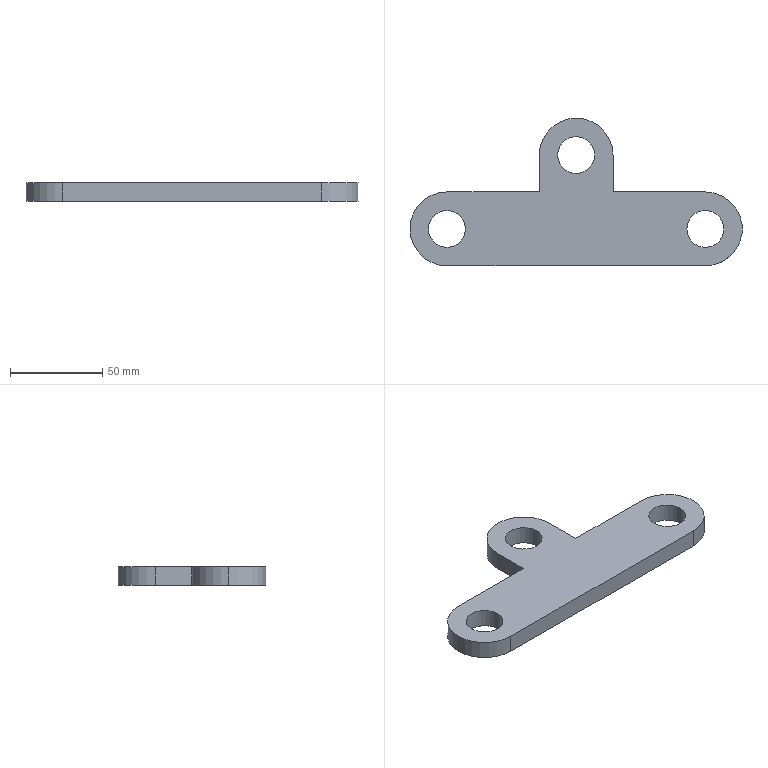Part | SolidWorks | features ICE 3, Extrusion 1, Fillet 1 | 1 solid | 18 faces | box 180 x 80 x 10 mm | volume 73425 mm3 | cylinder 11 | plane 7 | commonest cylinder face diameters 20 x6 40 x5
STEP:
#1=CARTESIAN_POINT('',(-10.,40.,0.));
#2=VERTEX_POINT('',#1);
#3=CARTESIAN_POINT('',(10.,40.,0.));
#4=VERTEX_POINT('',#3);
#5=CARTESIAN_POINT('',(0.,40.,0.));
#6=DIRECTION('',(0.,0.,1.));
#7=DIRECTION('',(1.,0.,0.));
#8=AXIS2_PLACEMENT_3D('',#5,#6,#7);
#9=CIRCLE('',#8,10.);
#10=EDGE_CURVE('',#2,#4,#9,.T.);
#11=ORIENTED_EDGE('',*,*,#10,.F.);
#12=CARTESIAN_POINT('',(-10.,40.,10.));
#13=VERTEX_POINT('',#12);
#14=CARTESIAN_POINT('',(-10.,40.,0.));
#15=DIRECTION('',(0.,0.,1.));
#16=VECTOR('',#15,1000.);
#17=LINE('',#14,#16);
#18=EDGE_CURVE('',#2,#13,#17,.T.);
#19=ORIENTED_EDGE('',*,*,#18,.T.);
#20=CARTESIAN_POINT('',(10.,40.,10.));
#21=VERTEX_POINT('',#20);
#22=CARTESIAN_POINT('',(0.,40.,10.));
#23=DIRECTION('',(0.,0.,1.));
#24=DIRECTION('',(1.,0.,0.));
#25=AXIS2_PLACEMENT_3D('',#22,#23,#24);
#26=CIRCLE('',#25,10.);
#27=EDGE_CURVE('',#13,#21,#26,.T.);
#28=ORIENTED_EDGE('',*,*,#27,.T.);
#29=CARTESIAN_POINT('',(10.,40.,0.));
#30=DIRECTION('',(0.,0.,1.));
#31=VECTOR('',#30,1000.);
#32=LINE('',#29,#31);
#33=EDGE_CURVE('',#4,#21,#32,.T.);
#34=ORIENTED_EDGE('',*,*,#33,.F.);
#35=EDGE_LOOP('',(#11,#19,#28,#34));
#36=FACE_OUTER_BOUND('',#35,.T.);
#37=CARTESIAN_POINT('',(0.,40.,0.));
#38=DIRECTION('',(0.,0.,1.));
#39=DIRECTION('',(1.,0.,0.));
#40=AXIS2_PLACEMENT_3D('',#37,#38,#39);
#41=CYLINDRICAL_SURFACE('',#40,10.);
#42=ADVANCED_FACE('',(#36),#41,.F.);
#43=CARTESIAN_POINT('',(-80.,0.,0.));
#44=VERTEX_POINT('',#43);
#45=CARTESIAN_POINT('',(-60.,0.,0.));
#46=VERTEX_POINT('',#45);
#47=CARTESIAN_POINT('',(-70.,0.,0.));
#48=DIRECTION('',(0.,0.,1.));
#49=DIRECTION('',(1.,0.,0.));
#50=AXIS2_PLACEMENT_3D('',#47,#48,#49);
#51=CIRCLE('',#50,10.);
#52=EDGE_CURVE('',#44,#46,#51,.T.);
#53=ORIENTED_EDGE('',*,*,#52,.F.);
#54=CARTESIAN_POINT('',(-80.,0.,10.));
#55=VERTEX_POINT('',#54);
#56=CARTESIAN_POINT('',(-80.,0.,0.));
#57=DIRECTION('',(0.,0.,1.));
#58=VECTOR('',#57,1000.);
#59=LINE('',#56,#58);
#60=EDGE_CURVE('',#44,#55,#59,.T.);
#61=ORIENTED_EDGE('',*,*,#60,.T.);
#62=CARTESIAN_POINT('',(-60.,0.,10.));
#63=VERTEX_POINT('',#62);
#64=CARTESIAN_POINT('',(-70.,0.,10.));
#65=DIRECTION('',(0.,0.,1.));
#66=DIRECTION('',(1.,0.,0.));
#67=AXIS2_PLACEMENT_3D('',#64,#65,#66);
#68=CIRCLE('',#67,10.);
#69=EDGE_CURVE('',#55,#63,#68,.T.);
#70=ORIENTED_EDGE('',*,*,#69,.T.);
#71=CARTESIAN_POINT('',(-60.,0.,0.));
#72=DIRECTION('',(0.,0.,1.));
#73=VECTOR('',#72,1000.);
#74=LINE('',#71,#73);
#75=EDGE_CURVE('',#46,#63,#74,.T.);
#76=ORIENTED_EDGE('',*,*,#75,.F.);
#77=EDGE_LOOP('',(#53,#61,#70,#76));
#78=FACE_OUTER_BOUND('',#77,.T.);
#79=CARTESIAN_POINT('',(-70.,0.,0.));
#80=DIRECTION('',(0.,0.,1.));
#81=DIRECTION('',(1.,0.,0.));
#82=AXIS2_PLACEMENT_3D('',#79,#80,#81);
#83=CYLINDRICAL_SURFACE('',#82,10.);
#84=ADVANCED_FACE('',(#78),#83,.F.);
#85=CARTESIAN_POINT('',(60.,0.,0.));
#86=VERTEX_POINT('',#85);
#87=CARTESIAN_POINT('',(80.,0.,0.));
#88=VERTEX_POINT('',#87);
#89=CARTESIAN_POINT('',(70.,0.,0.));
#90=DIRECTION('',(0.,0.,1.));
#91=DIRECTION('',(1.,0.,0.));
#92=AXIS2_PLACEMENT_3D('',#89,#90,#91);
#93=CIRCLE('',#92,10.);
#94=EDGE_CURVE('',#86,#88,#93,.T.);
#95=ORIENTED_EDGE('',*,*,#94,.F.);
#96=CARTESIAN_POINT('',(60.,0.,10.));
#97=VERTEX_POINT('',#96);
#98=CARTESIAN_POINT('',(60.,0.,0.));
#99=DIRECTION('',(0.,0.,1.));
#100=VECTOR('',#99,1000.);
#101=LINE('',#98,#100);
#102=EDGE_CURVE('',#86,#97,#101,.T.);
#103=ORIENTED_EDGE('',*,*,#102,.T.);
#104=CARTESIAN_POINT('',(80.,0.,10.));
#105=VERTEX_POINT('',#104);
#106=CARTESIAN_POINT('',(70.,0.,10.));
#107=DIRECTION('',(0.,0.,1.));
#108=DIRECTION('',(1.,0.,0.));
#109=AXIS2_PLACEMENT_3D('',#106,#107,#108);
#110=CIRCLE('',#109,10.);
#111=EDGE_CURVE('',#97,#105,#110,.T.);
#112=ORIENTED_EDGE('',*,*,#111,.T.);
#113=CARTESIAN_POINT('',(80.,0.,0.));
#114=DIRECTION('',(0.,0.,1.));
#115=VECTOR('',#114,1000.);
#116=LINE('',#113,#115);
#117=EDGE_CURVE('',#88,#105,#116,.T.);
#118=ORIENTED_EDGE('',*,*,#117,.F.);
#119=EDGE_LOOP('',(#95,#103,#112,#118));
#120=FACE_OUTER_BOUND('',#119,.T.);
#121=CARTESIAN_POINT('',(70.,0.,0.));
#122=DIRECTION('',(0.,0.,1.));
#123=DIRECTION('',(1.,0.,0.));
#124=AXIS2_PLACEMENT_3D('',#121,#122,#123);
#125=CYLINDRICAL_SURFACE('',#124,10.);
#126=ADVANCED_FACE('',(#120),#125,.F.);
#127=CARTESIAN_POINT('',(-90.,0.,10.));
#128=VERTEX_POINT('',#127);
#129=CARTESIAN_POINT('',(-70.,-20.,10.));
#130=VERTEX_POINT('',#129);
#131=CARTESIAN_POINT('',(-70.,0.,10.));
#132=DIRECTION('',(0.,0.,1.));
#133=DIRECTION('',(1.,0.,0.));
#134=AXIS2_PLACEMENT_3D('',#131,#132,#133);
#135=CIRCLE('',#134,20.);
#136=EDGE_CURVE('',#128,#130,#135,.T.);
#137=ORIENTED_EDGE('',*,*,#136,.F.);
#138=CARTESIAN_POINT('',(-90.,0.,0.));
#139=VERTEX_POINT('',#138);
#140=CARTESIAN_POINT('',(-90.,0.,10.));
#141=DIRECTION('',(0.,0.,-1.));
#142=VECTOR('',#141,1000.);
#143=LINE('',#140,#142);
#144=EDGE_CURVE('',#128,#139,#143,.T.);
#145=ORIENTED_EDGE('',*,*,#144,.T.);
#146=CARTESIAN_POINT('',(-70.,-20.,0.));
#147=VERTEX_POINT('',#146);
#148=CARTESIAN_POINT('',(-70.,0.,0.));
#149=DIRECTION('',(0.,0.,1.));
#150=DIRECTION('',(1.,0.,0.));
#151=AXIS2_PLACEMENT_3D('',#148,#149,#150);
#152=CIRCLE('',#151,20.);
#153=EDGE_CURVE('',#139,#147,#152,.T.);
#154=ORIENTED_EDGE('',*,*,#153,.T.);
#155=CARTESIAN_POINT('',(-70.,-20.,10.));
#156=DIRECTION('',(0.,0.,-1.));
#157=VECTOR('',#156,1000.);
#158=LINE('',#155,#157);
#159=EDGE_CURVE('',#130,#147,#158,.T.);
#160=ORIENTED_EDGE('',*,*,#159,.F.);
#161=EDGE_LOOP('',(#137,#145,#154,#160));
#162=FACE_OUTER_BOUND('',#161,.T.);
#163=CARTESIAN_POINT('',(-70.,0.,10.));
#164=DIRECTION('',(0.,0.,-1.));
#165=DIRECTION('',(-1.,0.,0.));
#166=AXIS2_PLACEMENT_3D('',#163,#164,#165);
#167=CYLINDRICAL_SURFACE('',#166,20.);
#168=ADVANCED_FACE('',(#162),#167,.T.);
#169=CARTESIAN_POINT('',(70.,20.,0.));
#170=VERTEX_POINT('',#169);
#171=CARTESIAN_POINT('',(20.,20.,0.));
#172=VERTEX_POINT('',#171);
#173=CARTESIAN_POINT('',(-70.,20.,0.));
#174=DIRECTION('',(-1.,0.,0.));
#175=VECTOR('',#174,1000.);
#176=LINE('',#173,#175);
#177=EDGE_CURVE('',#170,#172,#176,.T.);
#178=ORIENTED_EDGE('',*,*,#177,.T.);
#179=CARTESIAN_POINT('',(20.,20.,10.));
#180=VERTEX_POINT('',#179);
#181=CARTESIAN_POINT('',(20.,20.,0.));
#182=DIRECTION('',(0.,0.,1.));
#183=VECTOR('',#182,1000.);
#184=LINE('',#181,#183);
#185=EDGE_CURVE('',#172,#180,#184,.T.);
#186=ORIENTED_EDGE('',*,*,#185,.T.);
#187=CARTESIAN_POINT('',(70.,20.,10.));
#188=VERTEX_POINT('',#187);
#189=CARTESIAN_POINT('',(-70.,20.,10.));
#190=DIRECTION('',(-1.,0.,0.));
#191=VECTOR('',#190,1000.);
#192=LINE('',#189,#191);
#193=EDGE_CURVE('',#188,#180,#192,.T.);
#194=ORIENTED_EDGE('',*,*,#193,.F.);
#195=CARTESIAN_POINT('',(70.,20.,10.));
#196=DIRECTION('',(0.,0.,-1.));
#197=VECTOR('',#196,1000.);
#198=LINE('',#195,#197);
#199=EDGE_CURVE('',#188,#170,#198,.T.);
#200=ORIENTED_EDGE('',*,*,#199,.T.);
#201=EDGE_LOOP('',(#178,#186,#194,#200));
#202=FACE_OUTER_BOUND('',#201,.T.);
#203=CARTESIAN_POINT('',(-70.,20.,10.));
#204=DIRECTION('',(0.,-1.,0.));
#205=DIRECTION('',(0.,0.,-1.));
#206=AXIS2_PLACEMENT_3D('',#203,#204,#205);
#207=PLANE('',#206);
#208=ADVANCED_FACE('',(#202),#207,.F.);
#209=ORIENTED_EDGE('',*,*,#144,.F.);
#210=CARTESIAN_POINT('',(-70.,20.,10.));
#211=VERTEX_POINT('',#210);
#212=CARTESIAN_POINT('',(-70.,0.,10.));
#213=DIRECTION('',(0.,0.,1.));
#214=DIRECTION('',(1.,0.,0.));
#215=AXIS2_PLACEMENT_3D('',#212,#213,#214);
#216=CIRCLE('',#215,20.);
#217=EDGE_CURVE('',#211,#128,#216,.T.);
#218=ORIENTED_EDGE('',*,*,#217,.F.);
#219=CARTESIAN_POINT('',(-70.,20.,0.));
#220=VERTEX_POINT('',#219);
#221=CARTESIAN_POINT('',(-70.,20.,10.));
#222=DIRECTION('',(0.,0.,-1.));
#223=VECTOR('',#222,1000.);
#224=LINE('',#221,#223);
#225=EDGE_CURVE('',#211,#220,#224,.T.);
#226=ORIENTED_EDGE('',*,*,#225,.T.);
#227=CARTESIAN_POINT('',(-70.,0.,0.));
#228=DIRECTION('',(0.,0.,1.));
#229=DIRECTION('',(1.,0.,0.));
#230=AXIS2_PLACEMENT_3D('',#227,#228,#229);
#231=CIRCLE('',#230,20.);
#232=EDGE_CURVE('',#220,#139,#231,.T.);
#233=ORIENTED_EDGE('',*,*,#232,.T.);
#234=EDGE_LOOP('',(#209,#218,#226,#233));
#235=FACE_OUTER_BOUND('',#234,.T.);
#236=CARTESIAN_POINT('',(-70.,0.,10.));
#237=DIRECTION('',(0.,0.,-1.));
#238=DIRECTION('',(-1.,0.,0.));
#239=AXIS2_PLACEMENT_3D('',#236,#237,#238);
#240=CYLINDRICAL_SURFACE('',#239,20.);
#241=ADVANCED_FACE('',(#235),#240,.T.);
#242=CARTESIAN_POINT('',(70.,-20.,0.));
#243=VERTEX_POINT('',#242);
#244=CARTESIAN_POINT('',(-70.,-20.,0.));
#245=DIRECTION('',(1.,0.,0.));
#246=VECTOR('',#245,1000.);
#247=LINE('',#244,#246);
#248=EDGE_CURVE('',#147,#243,#247,.T.);
#249=ORIENTED_EDGE('',*,*,#248,.T.);
#250=CARTESIAN_POINT('',(70.,-20.,10.));
#251=VERTEX_POINT('',#250);
#252=CARTESIAN_POINT('',(70.,-20.,10.));
#253=DIRECTION('',(0.,0.,-1.));
#254=VECTOR('',#253,1000.);
#255=LINE('',#252,#254);
#256=EDGE_CURVE('',#251,#243,#255,.T.);
#257=ORIENTED_EDGE('',*,*,#256,.F.);
#258=CARTESIAN_POINT('',(-70.,-20.,10.));
#259=DIRECTION('',(1.,0.,0.));
#260=VECTOR('',#259,1000.);
#261=LINE('',#258,#260);
#262=EDGE_CURVE('',#130,#251,#261,.T.);
#263=ORIENTED_EDGE('',*,*,#262,.F.);
#264=ORIENTED_EDGE('',*,*,#159,.T.);
#265=EDGE_LOOP('',(#249,#257,#263,#264));
#266=FACE_OUTER_BOUND('',#265,.T.);
#267=CARTESIAN_POINT('',(-70.,-20.,10.));
#268=DIRECTION('',(0.,1.,0.));
#269=DIRECTION('',(0.,0.,1.));
#270=AXIS2_PLACEMENT_3D('',#267,#268,#269);
#271=PLANE('',#270);
#272=ADVANCED_FACE('',(#266),#271,.F.);
#273=CARTESIAN_POINT('',(70.,0.,0.));
#274=DIRECTION('',(0.,0.,1.));
#275=DIRECTION('',(1.,0.,0.));
#276=AXIS2_PLACEMENT_3D('',#273,#274,#275);
#277=CIRCLE('',#276,20.);
#278=EDGE_CURVE('',#243,#170,#277,.T.);
#279=ORIENTED_EDGE('',*,*,#278,.T.);
#280=ORIENTED_EDGE('',*,*,#199,.F.);
#281=CARTESIAN_POINT('',(70.,0.,10.));
#282=DIRECTION('',(0.,0.,1.));
#283=DIRECTION('',(1.,0.,0.));
#284=AXIS2_PLACEMENT_3D('',#281,#282,#283);
#285=CIRCLE('',#284,20.);
#286=EDGE_CURVE('',#251,#188,#285,.T.);
#287=ORIENTED_EDGE('',*,*,#286,.F.);
#288=ORIENTED_EDGE('',*,*,#256,.T.);
#289=EDGE_LOOP('',(#279,#280,#287,#288));
#290=FACE_OUTER_BOUND('',#289,.T.);
#291=CARTESIAN_POINT('',(70.,0.,10.));
#292=DIRECTION('',(0.,0.,-1.));
#293=DIRECTION('',(-1.,0.,0.));
#294=AXIS2_PLACEMENT_3D('',#291,#292,#293);
#295=CYLINDRICAL_SURFACE('',#294,20.);
#296=ADVANCED_FACE('',(#290),#295,.T.);
#297=CARTESIAN_POINT('',(-20.,20.,10.));
#298=VERTEX_POINT('',#297);
#299=CARTESIAN_POINT('',(-70.,20.,10.));
#300=DIRECTION('',(-1.,0.,0.));
#301=VECTOR('',#300,1000.);
#302=LINE('',#299,#301);
#303=EDGE_CURVE('',#298,#211,#302,.T.);
#304=ORIENTED_EDGE('',*,*,#303,.F.);
#305=CARTESIAN_POINT('',(-20.,20.,0.));
#306=VERTEX_POINT('',#305);
#307=CARTESIAN_POINT('',(-20.,20.,0.));
#308=DIRECTION('',(0.,0.,1.));
#309=VECTOR('',#308,1000.);
#310=LINE('',#307,#309);
#311=EDGE_CURVE('',#306,#298,#310,.T.);
#312=ORIENTED_EDGE('',*,*,#311,.F.);
#313=CARTESIAN_POINT('',(-70.,20.,0.));
#314=DIRECTION('',(-1.,0.,0.));
#315=VECTOR('',#314,1000.);
#316=LINE('',#313,#315);
#317=EDGE_CURVE('',#306,#220,#316,.T.);
#318=ORIENTED_EDGE('',*,*,#317,.T.);
#319=ORIENTED_EDGE('',*,*,#225,.F.);
#320=EDGE_LOOP('',(#304,#312,#318,#319));
#321=FACE_OUTER_BOUND('',#320,.T.);
#322=CARTESIAN_POINT('',(-70.,20.,10.));
#323=DIRECTION('',(0.,-1.,0.));
#324=DIRECTION('',(0.,0.,-1.));
#325=AXIS2_PLACEMENT_3D('',#322,#323,#324);
#326=PLANE('',#325);
#327=ADVANCED_FACE('',(#321),#326,.F.);
#328=CARTESIAN_POINT('',(0.,40.,10.));
#329=DIRECTION('',(0.,0.,1.));
#330=DIRECTION('',(1.,0.,0.));
#331=AXIS2_PLACEMENT_3D('',#328,#329,#330);
#332=CIRCLE('',#331,10.);
#333=EDGE_CURVE('',#21,#13,#332,.T.);
#334=ORIENTED_EDGE('',*,*,#333,.F.);
#335=ORIENTED_EDGE('',*,*,#27,.F.);
#336=EDGE_LOOP('',(#334,#335));
#337=FACE_BOUND('',#336,.T.);
#338=CARTESIAN_POINT('',(-70.,0.,10.));
#339=DIRECTION('',(0.,0.,1.));
#340=DIRECTION('',(1.,0.,0.));
#341=AXIS2_PLACEMENT_3D('',#338,#339,#340);
#342=CIRCLE('',#341,10.);
#343=EDGE_CURVE('',#63,#55,#342,.T.);
#344=ORIENTED_EDGE('',*,*,#343,.F.);
#345=ORIENTED_EDGE('',*,*,#69,.F.);
#346=EDGE_LOOP('',(#344,#345));
#347=FACE_BOUND('',#346,.T.);
#348=CARTESIAN_POINT('',(70.,0.,10.));
#349=DIRECTION('',(0.,0.,1.));
#350=DIRECTION('',(1.,0.,0.));
#351=AXIS2_PLACEMENT_3D('',#348,#349,#350);
#352=CIRCLE('',#351,10.);
#353=EDGE_CURVE('',#105,#97,#352,.T.);
#354=ORIENTED_EDGE('',*,*,#353,.F.);
#355=ORIENTED_EDGE('',*,*,#111,.F.);
#356=EDGE_LOOP('',(#354,#355));
#357=FACE_BOUND('',#356,.T.);
#358=CARTESIAN_POINT('',(20.,40.,10.));
#359=VERTEX_POINT('',#358);
#360=CARTESIAN_POINT('',(20.,60.,10.));
#361=DIRECTION('',(0.,1.,0.));
#362=VECTOR('',#361,1000.);
#363=LINE('',#360,#362);
#364=EDGE_CURVE('',#180,#359,#363,.T.);
#365=ORIENTED_EDGE('',*,*,#364,.T.);
#366=CARTESIAN_POINT('',(0.,60.,10.));
#367=VERTEX_POINT('',#366);
#368=CARTESIAN_POINT('',(0.,40.,10.));
#369=DIRECTION('',(0.,0.,1.));
#370=DIRECTION('',(1.,0.,0.));
#371=AXIS2_PLACEMENT_3D('',#368,#369,#370);
#372=CIRCLE('',#371,20.);
#373=EDGE_CURVE('',#359,#367,#372,.T.);
#374=ORIENTED_EDGE('',*,*,#373,.T.);
#375=CARTESIAN_POINT('',(-20.,40.,10.));
#376=VERTEX_POINT('',#375);
#377=CARTESIAN_POINT('',(0.,40.,10.));
#378=DIRECTION('',(0.,0.,1.));
#379=DIRECTION('',(1.,0.,0.));
#380=AXIS2_PLACEMENT_3D('',#377,#378,#379);
#381=CIRCLE('',#380,20.);
#382=EDGE_CURVE('',#367,#376,#381,.T.);
#383=ORIENTED_EDGE('',*,*,#382,.T.);
#384=CARTESIAN_POINT('',(-20.,20.,10.));
#385=DIRECTION('',(0.,-1.,0.));
#386=VECTOR('',#385,1000.);
#387=LINE('',#384,#386);
#388=EDGE_CURVE('',#376,#298,#387,.T.);
#389=ORIENTED_EDGE('',*,*,#388,.T.);
#390=ORIENTED_EDGE('',*,*,#303,.T.);
#391=ORIENTED_EDGE('',*,*,#217,.T.);
#392=ORIENTED_EDGE('',*,*,#136,.T.);
#393=ORIENTED_EDGE('',*,*,#262,.T.);
#394=ORIENTED_EDGE('',*,*,#286,.T.);
#395=ORIENTED_EDGE('',*,*,#193,.T.);
#396=EDGE_LOOP('',(#365,#374,#383,#389,#390,#391,#392,#393,#394,#395));
#397=FACE_OUTER_BOUND('',#396,.T.);
#398=CARTESIAN_POINT('',(-70.,0.,10.));
#399=DIRECTION('',(0.,0.,1.));
#400=DIRECTION('',(1.,0.,0.));
#401=AXIS2_PLACEMENT_3D('',#398,#399,#400);
#402=PLANE('',#401);
#403=ADVANCED_FACE('',(#337,#347,#357,#397),#402,.T.);
#404=CARTESIAN_POINT('',(0.,40.,0.));
#405=DIRECTION('',(0.,0.,1.));
#406=DIRECTION('',(1.,0.,0.));
#407=AXIS2_PLACEMENT_3D('',#404,#405,#406);
#408=CIRCLE('',#407,10.);
#409=EDGE_CURVE('',#4,#2,#408,.T.);
#410=ORIENTED_EDGE('',*,*,#409,.T.);
#411=ORIENTED_EDGE('',*,*,#10,.T.);
#412=EDGE_LOOP('',(#410,#411));
#413=FACE_BOUND('',#412,.T.);
#414=CARTESIAN_POINT('',(-70.,0.,0.));
#415=DIRECTION('',(0.,0.,1.));
#416=DIRECTION('',(1.,0.,0.));
#417=AXIS2_PLACEMENT_3D('',#414,#415,#416);
#418=CIRCLE('',#417,10.);
#419=EDGE_CURVE('',#46,#44,#418,.T.);
#420=ORIENTED_EDGE('',*,*,#419,.T.);
#421=ORIENTED_EDGE('',*,*,#52,.T.);
#422=EDGE_LOOP('',(#420,#421));
#423=FACE_BOUND('',#422,.T.);
#424=CARTESIAN_POINT('',(70.,0.,0.));
#425=DIRECTION('',(0.,0.,1.));
#426=DIRECTION('',(1.,0.,0.));
#427=AXIS2_PLACEMENT_3D('',#424,#425,#426);
#428=CIRCLE('',#427,10.);
#429=EDGE_CURVE('',#88,#86,#428,.T.);
#430=ORIENTED_EDGE('',*,*,#429,.T.);
#431=ORIENTED_EDGE('',*,*,#94,.T.);
#432=EDGE_LOOP('',(#430,#431));
#433=FACE_BOUND('',#432,.T.);
#434=CARTESIAN_POINT('',(-20.,40.,0.));
#435=VERTEX_POINT('',#434);
#436=CARTESIAN_POINT('',(0.,60.,0.));
#437=VERTEX_POINT('',#436);
#438=CARTESIAN_POINT('',(0.,40.,0.));
#439=DIRECTION('',(0.,0.,-1.));
#440=DIRECTION('',(1.,0.,0.));
#441=AXIS2_PLACEMENT_3D('',#438,#439,#440);
#442=CIRCLE('',#441,20.);
#443=EDGE_CURVE('',#435,#437,#442,.T.);
#444=ORIENTED_EDGE('',*,*,#443,.T.);
#445=CARTESIAN_POINT('',(20.,40.,0.));
#446=VERTEX_POINT('',#445);
#447=CARTESIAN_POINT('',(0.,40.,0.));
#448=DIRECTION('',(0.,0.,-1.));
#449=DIRECTION('',(1.,0.,0.));
#450=AXIS2_PLACEMENT_3D('',#447,#448,#449);
#451=CIRCLE('',#450,20.);
#452=EDGE_CURVE('',#437,#446,#451,.T.);
#453=ORIENTED_EDGE('',*,*,#452,.T.);
#454=CARTESIAN_POINT('',(20.,60.,0.));
#455=DIRECTION('',(0.,1.,0.));
#456=VECTOR('',#455,1000.);
#457=LINE('',#454,#456);
#458=EDGE_CURVE('',#172,#446,#457,.T.);
#459=ORIENTED_EDGE('',*,*,#458,.F.);
#460=ORIENTED_EDGE('',*,*,#177,.F.);
#461=ORIENTED_EDGE('',*,*,#278,.F.);
#462=ORIENTED_EDGE('',*,*,#248,.F.);
#463=ORIENTED_EDGE('',*,*,#153,.F.);
#464=ORIENTED_EDGE('',*,*,#232,.F.);
#465=ORIENTED_EDGE('',*,*,#317,.F.);
#466=CARTESIAN_POINT('',(-20.,20.,0.));
#467=DIRECTION('',(0.,-1.,0.));
#468=VECTOR('',#467,1000.);
#469=LINE('',#466,#468);
#470=EDGE_CURVE('',#435,#306,#469,.T.);
#471=ORIENTED_EDGE('',*,*,#470,.F.);
#472=EDGE_LOOP('',(#444,#453,#459,#460,#461,#462,#463,#464,#465,#471));
#473=FACE_OUTER_BOUND('',#472,.T.);
#474=CARTESIAN_POINT('',(-70.,0.,0.));
#475=DIRECTION('',(0.,0.,1.));
#476=DIRECTION('',(1.,0.,0.));
#477=AXIS2_PLACEMENT_3D('',#474,#475,#476);
#478=PLANE('',#477);
#479=ADVANCED_FACE('',(#413,#423,#433,#473),#478,.F.);
#480=ORIENTED_EDGE('',*,*,#102,.F.);
#481=ORIENTED_EDGE('',*,*,#429,.F.);
#482=ORIENTED_EDGE('',*,*,#117,.T.);
#483=ORIENTED_EDGE('',*,*,#353,.T.);
#484=EDGE_LOOP('',(#480,#481,#482,#483));
#485=FACE_OUTER_BOUND('',#484,.T.);
#486=CARTESIAN_POINT('',(70.,0.,0.));
#487=DIRECTION('',(0.,0.,1.));
#488=DIRECTION('',(1.,0.,0.));
#489=AXIS2_PLACEMENT_3D('',#486,#487,#488);
#490=CYLINDRICAL_SURFACE('',#489,10.);
#491=ADVANCED_FACE('',(#485),#490,.F.);
#492=ORIENTED_EDGE('',*,*,#60,.F.);
#493=ORIENTED_EDGE('',*,*,#419,.F.);
#494=ORIENTED_EDGE('',*,*,#75,.T.);
#495=ORIENTED_EDGE('',*,*,#343,.T.);
#496=EDGE_LOOP('',(#492,#493,#494,#495));
#497=FACE_OUTER_BOUND('',#496,.T.);
#498=CARTESIAN_POINT('',(-70.,0.,0.));
#499=DIRECTION('',(0.,0.,1.));
#500=DIRECTION('',(1.,0.,0.));
#501=AXIS2_PLACEMENT_3D('',#498,#499,#500);
#502=CYLINDRICAL_SURFACE('',#501,10.);
#503=ADVANCED_FACE('',(#497),#502,.F.);
#504=ORIENTED_EDGE('',*,*,#458,.T.);
#505=CARTESIAN_POINT('',(20.,40.,0.));
#506=DIRECTION('',(0.,0.,1.));
#507=VECTOR('',#506,1000.);
#508=LINE('',#505,#507);
#509=EDGE_CURVE('',#446,#359,#508,.T.);
#510=ORIENTED_EDGE('',*,*,#509,.T.);
#511=ORIENTED_EDGE('',*,*,#364,.F.);
#512=ORIENTED_EDGE('',*,*,#185,.F.);
#513=EDGE_LOOP('',(#504,#510,#511,#512));
#514=FACE_OUTER_BOUND('',#513,.T.);
#515=CARTESIAN_POINT('',(20.,60.,0.));
#516=DIRECTION('',(1.,0.,0.));
#517=DIRECTION('',(0.,0.,-1.));
#518=AXIS2_PLACEMENT_3D('',#515,#516,#517);
#519=PLANE('',#518);
#520=ADVANCED_FACE('',(#514),#519,.T.);
#521=ORIENTED_EDGE('',*,*,#388,.F.);
#522=CARTESIAN_POINT('',(-20.,40.,0.));
#523=DIRECTION('',(0.,0.,-1.));
#524=VECTOR('',#523,1000.);
#525=LINE('',#522,#524);
#526=EDGE_CURVE('',#376,#435,#525,.T.);
#527=ORIENTED_EDGE('',*,*,#526,.T.);
#528=ORIENTED_EDGE('',*,*,#470,.T.);
#529=ORIENTED_EDGE('',*,*,#311,.T.);
#530=EDGE_LOOP('',(#521,#527,#528,#529));
#531=FACE_OUTER_BOUND('',#530,.T.);
#532=CARTESIAN_POINT('',(-20.,20.,0.));
#533=DIRECTION('',(-1.,0.,0.));
#534=DIRECTION('',(0.,-1.,0.));
#535=AXIS2_PLACEMENT_3D('',#532,#533,#534);
#536=PLANE('',#535);
#537=ADVANCED_FACE('',(#531),#536,.T.);
#538=CARTESIAN_POINT('',(0.,60.,0.));
#539=DIRECTION('',(0.,0.,1.));
#540=VECTOR('',#539,1000.);
#541=LINE('',#538,#540);
#542=EDGE_CURVE('',#437,#367,#541,.T.);
#543=ORIENTED_EDGE('',*,*,#542,.F.);
#544=ORIENTED_EDGE('',*,*,#443,.F.);
#545=ORIENTED_EDGE('',*,*,#526,.F.);
#546=ORIENTED_EDGE('',*,*,#382,.F.);
#547=EDGE_LOOP('',(#543,#544,#545,#546));
#548=FACE_OUTER_BOUND('',#547,.T.);
#549=CARTESIAN_POINT('',(0.,40.,0.));
#550=DIRECTION('',(0.,0.,1.));
#551=DIRECTION('',(1.,0.,0.));
#552=AXIS2_PLACEMENT_3D('',#549,#550,#551);
#553=CYLINDRICAL_SURFACE('',#552,20.);
#554=ADVANCED_FACE('',(#548),#553,.T.);
#555=ORIENTED_EDGE('',*,*,#452,.F.);
#556=ORIENTED_EDGE('',*,*,#542,.T.);
#557=ORIENTED_EDGE('',*,*,#373,.F.);
#558=ORIENTED_EDGE('',*,*,#509,.F.);
#559=EDGE_LOOP('',(#555,#556,#557,#558));
#560=FACE_OUTER_BOUND('',#559,.T.);
#561=CARTESIAN_POINT('',(0.,40.,0.));
#562=DIRECTION('',(0.,0.,1.));
#563=DIRECTION('',(1.,0.,0.));
#564=AXIS2_PLACEMENT_3D('',#561,#562,#563);
#565=CYLINDRICAL_SURFACE('',#564,20.);
#566=ADVANCED_FACE('',(#560),#565,.T.);
#567=ORIENTED_EDGE('',*,*,#18,.F.);
#568=ORIENTED_EDGE('',*,*,#409,.F.);
#569=ORIENTED_EDGE('',*,*,#33,.T.);
#570=ORIENTED_EDGE('',*,*,#333,.T.);
#571=EDGE_LOOP('',(#567,#568,#569,#570));
#572=FACE_OUTER_BOUND('',#571,.T.);
#573=CARTESIAN_POINT('',(0.,40.,0.));
#574=DIRECTION('',(0.,0.,1.));
#575=DIRECTION('',(1.,0.,0.));
#576=AXIS2_PLACEMENT_3D('',#573,#574,#575);
#577=CYLINDRICAL_SURFACE('',#576,10.);
#578=ADVANCED_FACE('',(#572),#577,.F.);
#579=CLOSED_SHELL('',(#42,#84,#126,#168,#208,#241,#272,#296,#327,#403,#479,#491,#503,#520,#537,#554,#566,#578));
#580=MANIFOLD_SOLID_BREP('',#579);
#581=CARTESIAN_POINT('',(0.,0.,0.));
#582=DIRECTION('',(0.,0.,1.));
#583=DIRECTION('',(1.,0.,0.));
#584=AXIS2_PLACEMENT_3D('',#581,#582,#583);
#585=(LENGTH_UNIT()NAMED_UNIT(*)SI_UNIT(.MILLI.,.METRE.));
#586=UNCERTAINTY_MEASURE_WITH_UNIT(LENGTH_MEASURE(0.00001),#585,'','');
#587=(NAMED_UNIT(*)PLANE_ANGLE_UNIT()SI_UNIT($,.RADIAN.));
#588=(NAMED_UNIT(*)SI_UNIT($,.STERADIAN.)SOLID_ANGLE_UNIT());
#589=(GEOMETRIC_REPRESENTATION_CONTEXT(3)GLOBAL_UNCERTAINTY_ASSIGNED_CONTEXT((#586))GLOBAL_UNIT_ASSIGNED_CONTEXT((#585,#587,#588))REPRESENTATION_CONTEXT('',''));
#590=ADVANCED_BREP_SHAPE_REPRESENTATION('',(#580,#584),#589);